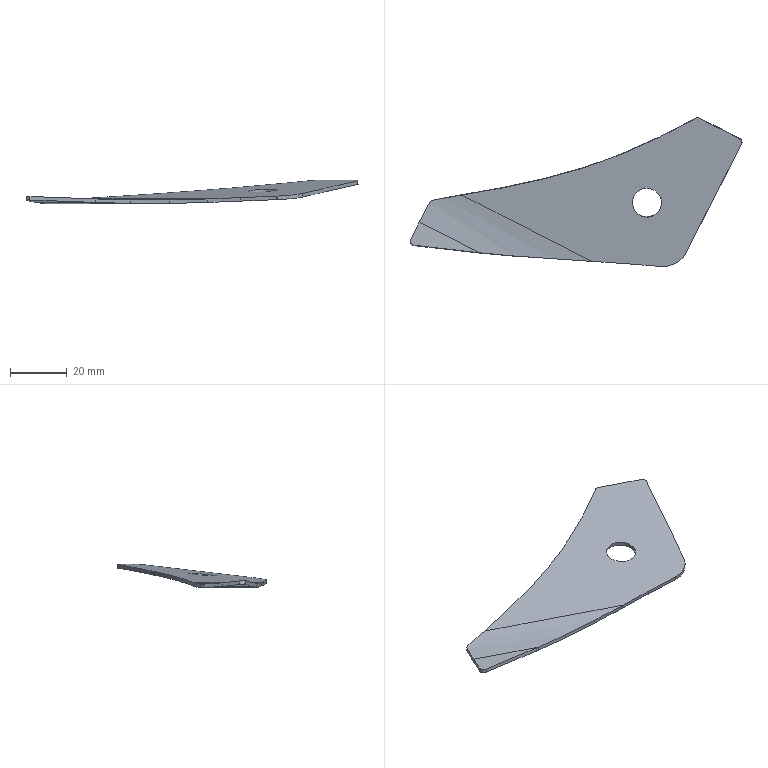Part | STEP file | gslz 2016.10.28-13_id1318_x_t | 1 solid | 26 faces | box 117.473 x 52.739 x 8.208 mm | volume 4131 mm3 | spline 10 | other 7 | cylinder 5 | plane 4 | commonest cylinder face diameters 10.3 x1 20.664 x1 146 x1 148.5 x1 33243 x1